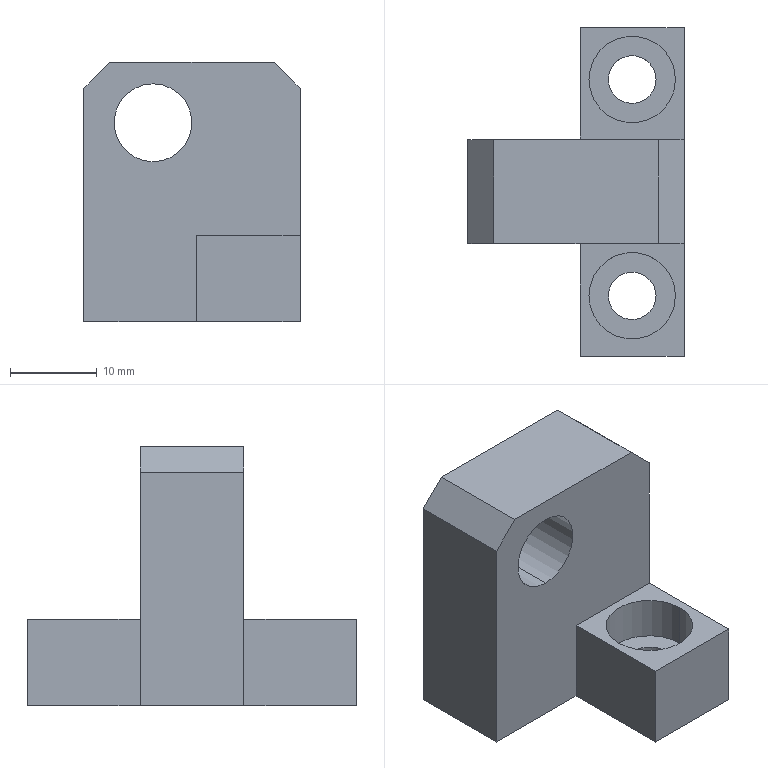Part | STEP file | 11-FG-E00411 | 1 solid | 26 faces | box 25 x 38 x 30 mm | volume 10226 mm3 | plane 16 | cylinder 10 | commonest cylinder face diameters 5.5 x4 10 x4 9 x2
STEP:
#1=CARTESIAN_POINT('',(-25.941,19.216,5.));
#2=VERTEX_POINT('',#1);
#3=CARTESIAN_POINT('',(-15.941,19.216,5.));
#4=VERTEX_POINT('',#3);
#5=CARTESIAN_POINT('',(-20.941,19.216,5.));
#6=DIRECTION('',(0.,0.,1.));
#7=DIRECTION('',(1.,0.,0.));
#8=AXIS2_PLACEMENT_3D('',#5,#6,#7);
#9=CIRCLE('',#8,5.);
#10=EDGE_CURVE('',#2,#4,#9,.T.);
#11=ORIENTED_EDGE('',*,*,#10,.F.);
#12=CARTESIAN_POINT('',(-25.941,19.216,10.));
#13=VERTEX_POINT('',#12);
#14=CARTESIAN_POINT('',(-25.941,19.216,10.));
#15=DIRECTION('',(0.,0.,1.));
#16=VECTOR('',#15,1000.);
#17=LINE('',#14,#16);
#18=EDGE_CURVE('',#2,#13,#17,.T.);
#19=ORIENTED_EDGE('',*,*,#18,.T.);
#20=CARTESIAN_POINT('',(-15.941,19.216,10.));
#21=VERTEX_POINT('',#20);
#22=CARTESIAN_POINT('',(-20.941,19.216,10.));
#23=DIRECTION('',(0.,0.,1.));
#24=DIRECTION('',(1.,0.,0.));
#25=AXIS2_PLACEMENT_3D('',#22,#23,#24);
#26=CIRCLE('',#25,5.);
#27=EDGE_CURVE('',#13,#21,#26,.T.);
#28=ORIENTED_EDGE('',*,*,#27,.T.);
#29=CARTESIAN_POINT('',(-15.941,19.216,10.));
#30=DIRECTION('',(0.,0.,1.));
#31=VECTOR('',#30,1000.);
#32=LINE('',#29,#31);
#33=EDGE_CURVE('',#4,#21,#32,.T.);
#34=ORIENTED_EDGE('',*,*,#33,.F.);
#35=EDGE_LOOP('',(#11,#19,#28,#34));
#36=FACE_OUTER_BOUND('',#35,.T.);
#37=CARTESIAN_POINT('',(-20.941,19.216,10.));
#38=DIRECTION('',(0.,0.,1.));
#39=DIRECTION('',(1.,0.,0.));
#40=AXIS2_PLACEMENT_3D('',#37,#38,#39);
#41=CYLINDRICAL_SURFACE('',#40,5.);
#42=ADVANCED_FACE('',(#36),#41,.F.);
#43=CARTESIAN_POINT('',(-23.691,19.216,0.));
#44=VERTEX_POINT('',#43);
#45=CARTESIAN_POINT('',(-18.191,19.216,0.));
#46=VERTEX_POINT('',#45);
#47=CARTESIAN_POINT('',(-20.941,19.216,0.));
#48=DIRECTION('',(0.,0.,1.));
#49=DIRECTION('',(1.,0.,0.));
#50=AXIS2_PLACEMENT_3D('',#47,#48,#49);
#51=CIRCLE('',#50,2.75);
#52=EDGE_CURVE('',#44,#46,#51,.T.);
#53=ORIENTED_EDGE('',*,*,#52,.F.);
#54=CARTESIAN_POINT('',(-23.691,19.216,5.));
#55=VERTEX_POINT('',#54);
#56=CARTESIAN_POINT('',(-23.691,19.216,10.));
#57=DIRECTION('',(0.,0.,1.));
#58=VECTOR('',#57,1000.);
#59=LINE('',#56,#58);
#60=EDGE_CURVE('',#44,#55,#59,.T.);
#61=ORIENTED_EDGE('',*,*,#60,.T.);
#62=CARTESIAN_POINT('',(-18.191,19.216,5.));
#63=VERTEX_POINT('',#62);
#64=CARTESIAN_POINT('',(-20.941,19.216,5.));
#65=DIRECTION('',(0.,0.,1.));
#66=DIRECTION('',(1.,0.,0.));
#67=AXIS2_PLACEMENT_3D('',#64,#65,#66);
#68=CIRCLE('',#67,2.75);
#69=EDGE_CURVE('',#55,#63,#68,.T.);
#70=ORIENTED_EDGE('',*,*,#69,.T.);
#71=CARTESIAN_POINT('',(-18.191,19.216,10.));
#72=DIRECTION('',(0.,0.,1.));
#73=VECTOR('',#72,1000.);
#74=LINE('',#71,#73);
#75=EDGE_CURVE('',#46,#63,#74,.T.);
#76=ORIENTED_EDGE('',*,*,#75,.F.);
#77=EDGE_LOOP('',(#53,#61,#70,#76));
#78=FACE_OUTER_BOUND('',#77,.T.);
#79=CARTESIAN_POINT('',(-20.941,19.216,10.));
#80=DIRECTION('',(0.,0.,1.));
#81=DIRECTION('',(1.,0.,0.));
#82=AXIS2_PLACEMENT_3D('',#79,#80,#81);
#83=CYLINDRICAL_SURFACE('',#82,2.75);
#84=ADVANCED_FACE('',(#78),#83,.F.);
#85=CARTESIAN_POINT('',(-25.941,-5.784,5.));
#86=VERTEX_POINT('',#85);
#87=CARTESIAN_POINT('',(-15.941,-5.784,5.));
#88=VERTEX_POINT('',#87);
#89=CARTESIAN_POINT('',(-20.941,-5.784,5.));
#90=DIRECTION('',(0.,0.,1.));
#91=DIRECTION('',(1.,0.,0.));
#92=AXIS2_PLACEMENT_3D('',#89,#90,#91);
#93=CIRCLE('',#92,5.);
#94=EDGE_CURVE('',#86,#88,#93,.T.);
#95=ORIENTED_EDGE('',*,*,#94,.F.);
#96=CARTESIAN_POINT('',(-25.941,-5.784,10.));
#97=VERTEX_POINT('',#96);
#98=CARTESIAN_POINT('',(-25.941,-5.784,10.));
#99=DIRECTION('',(0.,0.,1.));
#100=VECTOR('',#99,1000.);
#101=LINE('',#98,#100);
#102=EDGE_CURVE('',#86,#97,#101,.T.);
#103=ORIENTED_EDGE('',*,*,#102,.T.);
#104=CARTESIAN_POINT('',(-15.941,-5.784,10.));
#105=VERTEX_POINT('',#104);
#106=CARTESIAN_POINT('',(-20.941,-5.784,10.));
#107=DIRECTION('',(0.,0.,1.));
#108=DIRECTION('',(1.,0.,0.));
#109=AXIS2_PLACEMENT_3D('',#106,#107,#108);
#110=CIRCLE('',#109,5.);
#111=EDGE_CURVE('',#97,#105,#110,.T.);
#112=ORIENTED_EDGE('',*,*,#111,.T.);
#113=CARTESIAN_POINT('',(-15.941,-5.784,10.));
#114=DIRECTION('',(0.,0.,1.));
#115=VECTOR('',#114,1000.);
#116=LINE('',#113,#115);
#117=EDGE_CURVE('',#88,#105,#116,.T.);
#118=ORIENTED_EDGE('',*,*,#117,.F.);
#119=EDGE_LOOP('',(#95,#103,#112,#118));
#120=FACE_OUTER_BOUND('',#119,.T.);
#121=CARTESIAN_POINT('',(-20.941,-5.784,10.));
#122=DIRECTION('',(0.,0.,1.));
#123=DIRECTION('',(1.,0.,0.));
#124=AXIS2_PLACEMENT_3D('',#121,#122,#123);
#125=CYLINDRICAL_SURFACE('',#124,5.);
#126=ADVANCED_FACE('',(#120),#125,.F.);
#127=CARTESIAN_POINT('',(-23.691,-5.784,0.));
#128=VERTEX_POINT('',#127);
#129=CARTESIAN_POINT('',(-18.191,-5.784,0.));
#130=VERTEX_POINT('',#129);
#131=CARTESIAN_POINT('',(-20.941,-5.784,0.));
#132=DIRECTION('',(0.,0.,1.));
#133=DIRECTION('',(1.,0.,0.));
#134=AXIS2_PLACEMENT_3D('',#131,#132,#133);
#135=CIRCLE('',#134,2.75);
#136=EDGE_CURVE('',#128,#130,#135,.T.);
#137=ORIENTED_EDGE('',*,*,#136,.F.);
#138=CARTESIAN_POINT('',(-23.691,-5.784,5.));
#139=VERTEX_POINT('',#138);
#140=CARTESIAN_POINT('',(-23.691,-5.784,10.));
#141=DIRECTION('',(0.,0.,1.));
#142=VECTOR('',#141,1000.);
#143=LINE('',#140,#142);
#144=EDGE_CURVE('',#128,#139,#143,.T.);
#145=ORIENTED_EDGE('',*,*,#144,.T.);
#146=CARTESIAN_POINT('',(-18.191,-5.784,5.));
#147=VERTEX_POINT('',#146);
#148=CARTESIAN_POINT('',(-20.941,-5.784,5.));
#149=DIRECTION('',(0.,0.,1.));
#150=DIRECTION('',(1.,0.,0.));
#151=AXIS2_PLACEMENT_3D('',#148,#149,#150);
#152=CIRCLE('',#151,2.75);
#153=EDGE_CURVE('',#139,#147,#152,.T.);
#154=ORIENTED_EDGE('',*,*,#153,.T.);
#155=CARTESIAN_POINT('',(-18.191,-5.784,10.));
#156=DIRECTION('',(0.,0.,1.));
#157=VECTOR('',#156,1000.);
#158=LINE('',#155,#157);
#159=EDGE_CURVE('',#130,#147,#158,.T.);
#160=ORIENTED_EDGE('',*,*,#159,.F.);
#161=EDGE_LOOP('',(#137,#145,#154,#160));
#162=FACE_OUTER_BOUND('',#161,.T.);
#163=CARTESIAN_POINT('',(-20.941,-5.784,10.));
#164=DIRECTION('',(0.,0.,1.));
#165=DIRECTION('',(1.,0.,0.));
#166=AXIS2_PLACEMENT_3D('',#163,#164,#165);
#167=CYLINDRICAL_SURFACE('',#166,2.75);
#168=ADVANCED_FACE('',(#162),#167,.F.);
#169=CARTESIAN_POINT('',(-31.941,0.2155,18.5));
#170=VERTEX_POINT('',#169);
#171=CARTESIAN_POINT('',(-31.941,0.2155,27.5));
#172=VERTEX_POINT('',#171);
#173=CARTESIAN_POINT('',(-31.941,0.2155,23.));
#174=DIRECTION('',(0.,1.,0.));
#175=DIRECTION('',(-1.,0.,0.));
#176=AXIS2_PLACEMENT_3D('',#173,#174,#175);
#177=CIRCLE('',#176,4.5);
#178=EDGE_CURVE('',#170,#172,#177,.T.);
#179=ORIENTED_EDGE('',*,*,#178,.F.);
#180=CARTESIAN_POINT('',(-31.941,12.216,18.5));
#181=VERTEX_POINT('',#180);
#182=CARTESIAN_POINT('',(-31.941,12.216,18.5));
#183=DIRECTION('',(0.,1.,0.));
#184=VECTOR('',#183,1000.);
#185=LINE('',#182,#184);
#186=EDGE_CURVE('',#170,#181,#185,.T.);
#187=ORIENTED_EDGE('',*,*,#186,.T.);
#188=CARTESIAN_POINT('',(-31.941,12.216,27.5));
#189=VERTEX_POINT('',#188);
#190=CARTESIAN_POINT('',(-31.941,12.216,23.));
#191=DIRECTION('',(0.,1.,0.));
#192=DIRECTION('',(0.,0.,1.));
#193=AXIS2_PLACEMENT_3D('',#190,#191,#192);
#194=CIRCLE('',#193,4.5);
#195=EDGE_CURVE('',#181,#189,#194,.T.);
#196=ORIENTED_EDGE('',*,*,#195,.T.);
#197=CARTESIAN_POINT('',(-31.941,12.216,27.5));
#198=DIRECTION('',(0.,1.,0.));
#199=VECTOR('',#198,1000.);
#200=LINE('',#197,#199);
#201=EDGE_CURVE('',#172,#189,#200,.T.);
#202=ORIENTED_EDGE('',*,*,#201,.F.);
#203=EDGE_LOOP('',(#179,#187,#196,#202));
#204=FACE_OUTER_BOUND('',#203,.T.);
#205=CARTESIAN_POINT('',(-31.941,12.216,23.));
#206=DIRECTION('',(0.,1.,0.));
#207=DIRECTION('',(0.,0.,1.));
#208=AXIS2_PLACEMENT_3D('',#205,#206,#207);
#209=CYLINDRICAL_SURFACE('',#208,4.5);
#210=ADVANCED_FACE('',(#204),#209,.F.);
#211=CARTESIAN_POINT('',(-14.941,0.2155,10.));
#212=VERTEX_POINT('',#211);
#213=CARTESIAN_POINT('',(-26.941,0.2155,10.));
#214=VERTEX_POINT('',#213);
#215=CARTESIAN_POINT('',(-39.941,0.2155,10.));
#216=DIRECTION('',(-1.,0.,0.));
#217=VECTOR('',#216,1000.);
#218=LINE('',#215,#217);
#219=EDGE_CURVE('',#212,#214,#218,.T.);
#220=ORIENTED_EDGE('',*,*,#219,.T.);
#221=CARTESIAN_POINT('',(-26.941,-12.784,10.));
#222=VERTEX_POINT('',#221);
#223=CARTESIAN_POINT('',(-26.941,-24.784,10.));
#224=DIRECTION('',(0.,1.,0.));
#225=VECTOR('',#224,1000.);
#226=LINE('',#223,#225);
#227=EDGE_CURVE('',#222,#214,#226,.T.);
#228=ORIENTED_EDGE('',*,*,#227,.F.);
#229=CARTESIAN_POINT('',(-14.941,-12.784,10.));
#230=VERTEX_POINT('',#229);
#231=CARTESIAN_POINT('',(-14.941,-12.784,10.));
#232=DIRECTION('',(-1.,0.,0.));
#233=VECTOR('',#232,1000.);
#234=LINE('',#231,#233);
#235=EDGE_CURVE('',#230,#222,#234,.T.);
#236=ORIENTED_EDGE('',*,*,#235,.F.);
#237=CARTESIAN_POINT('',(-14.941,-24.784,10.));
#238=DIRECTION('',(0.,1.,0.));
#239=VECTOR('',#238,1000.);
#240=LINE('',#237,#239);
#241=EDGE_CURVE('',#230,#212,#240,.T.);
#242=ORIENTED_EDGE('',*,*,#241,.T.);
#243=EDGE_LOOP('',(#220,#228,#236,#242));
#244=FACE_OUTER_BOUND('',#243,.T.);
#245=CARTESIAN_POINT('',(-20.941,-5.784,10.));
#246=DIRECTION('',(0.,0.,1.));
#247=DIRECTION('',(1.,0.,0.));
#248=AXIS2_PLACEMENT_3D('',#245,#246,#247);
#249=CIRCLE('',#248,5.);
#250=EDGE_CURVE('',#105,#97,#249,.T.);
#251=ORIENTED_EDGE('',*,*,#250,.F.);
#252=ORIENTED_EDGE('',*,*,#111,.F.);
#253=EDGE_LOOP('',(#251,#252));
#254=FACE_BOUND('',#253,.T.);
#255=CARTESIAN_POINT('',(-39.941,0.2155,10.));
#256=DIRECTION('',(0.,0.,-1.));
#257=DIRECTION('',(-1.,0.,0.));
#258=AXIS2_PLACEMENT_3D('',#255,#256,#257);
#259=PLANE('',#258);
#260=ADVANCED_FACE('',(#244,#254),#259,.F.);
#261=CARTESIAN_POINT('',(-36.941,12.216,30.));
#262=VERTEX_POINT('',#261);
#263=CARTESIAN_POINT('',(-17.941,12.216,30.));
#264=VERTEX_POINT('',#263);
#265=CARTESIAN_POINT('',(-39.941,12.216,30.));
#266=DIRECTION('',(1.,0.,0.));
#267=VECTOR('',#266,1000.);
#268=LINE('',#265,#267);
#269=EDGE_CURVE('',#262,#264,#268,.T.);
#270=ORIENTED_EDGE('',*,*,#269,.T.);
#271=CARTESIAN_POINT('',(-14.941,12.216,27.));
#272=VERTEX_POINT('',#271);
#273=CARTESIAN_POINT('',(-17.941,12.216,30.));
#274=DIRECTION('',(0.7071,0.,-0.7071));
#275=VECTOR('',#274,1000.);
#276=LINE('',#273,#275);
#277=EDGE_CURVE('',#264,#272,#276,.T.);
#278=ORIENTED_EDGE('',*,*,#277,.T.);
#279=CARTESIAN_POINT('',(-14.941,12.216,10.));
#280=VERTEX_POINT('',#279);
#281=CARTESIAN_POINT('',(-14.941,12.216,10.));
#282=DIRECTION('',(0.,0.,1.));
#283=VECTOR('',#282,1000.);
#284=LINE('',#281,#283);
#285=EDGE_CURVE('',#280,#272,#284,.T.);
#286=ORIENTED_EDGE('',*,*,#285,.F.);
#287=CARTESIAN_POINT('',(-26.941,12.216,10.));
#288=VERTEX_POINT('',#287);
#289=CARTESIAN_POINT('',(-39.941,12.216,10.));
#290=DIRECTION('',(1.,0.,0.));
#291=VECTOR('',#290,1000.);
#292=LINE('',#289,#291);
#293=EDGE_CURVE('',#288,#280,#292,.T.);
#294=ORIENTED_EDGE('',*,*,#293,.F.);
#295=CARTESIAN_POINT('',(-26.941,12.216,0.));
#296=VERTEX_POINT('',#295);
#297=CARTESIAN_POINT('',(-26.941,12.216,0.));
#298=DIRECTION('',(0.,0.,1.));
#299=VECTOR('',#298,1000.);
#300=LINE('',#297,#299);
#301=EDGE_CURVE('',#296,#288,#300,.T.);
#302=ORIENTED_EDGE('',*,*,#301,.F.);
#303=CARTESIAN_POINT('',(-39.941,12.216,0.));
#304=VERTEX_POINT('',#303);
#305=CARTESIAN_POINT('',(-39.941,12.216,0.));
#306=DIRECTION('',(1.,0.,0.));
#307=VECTOR('',#306,1000.);
#308=LINE('',#305,#307);
#309=EDGE_CURVE('',#304,#296,#308,.T.);
#310=ORIENTED_EDGE('',*,*,#309,.F.);
#311=CARTESIAN_POINT('',(-39.941,12.216,27.));
#312=VERTEX_POINT('',#311);
#313=CARTESIAN_POINT('',(-39.941,12.216,10.));
#314=DIRECTION('',(0.,0.,1.));
#315=VECTOR('',#314,1000.);
#316=LINE('',#313,#315);
#317=EDGE_CURVE('',#304,#312,#316,.T.);
#318=ORIENTED_EDGE('',*,*,#317,.T.);
#319=CARTESIAN_POINT('',(-36.941,12.216,30.));
#320=DIRECTION('',(0.7071,0.,0.7071));
#321=VECTOR('',#320,1000.);
#322=LINE('',#319,#321);
#323=EDGE_CURVE('',#312,#262,#322,.T.);
#324=ORIENTED_EDGE('',*,*,#323,.T.);
#325=EDGE_LOOP('',(#270,#278,#286,#294,#302,#310,#318,#324));
#326=FACE_OUTER_BOUND('',#325,.T.);
#327=CARTESIAN_POINT('',(-31.941,12.216,23.));
#328=DIRECTION('',(0.,1.,0.));
#329=DIRECTION('',(0.,0.,1.));
#330=AXIS2_PLACEMENT_3D('',#327,#328,#329);
#331=CIRCLE('',#330,4.5);
#332=EDGE_CURVE('',#189,#181,#331,.T.);
#333=ORIENTED_EDGE('',*,*,#332,.F.);
#334=ORIENTED_EDGE('',*,*,#195,.F.);
#335=EDGE_LOOP('',(#333,#334));
#336=FACE_BOUND('',#335,.T.);
#337=CARTESIAN_POINT('',(-39.941,12.216,10.));
#338=DIRECTION('',(0.,-1.,0.));
#339=DIRECTION('',(0.,0.,-1.));
#340=AXIS2_PLACEMENT_3D('',#337,#338,#339);
#341=PLANE('',#340);
#342=ADVANCED_FACE('',(#326,#336),#341,.F.);
#343=CARTESIAN_POINT('',(-14.941,25.216,0.));
#344=VERTEX_POINT('',#343);
#345=CARTESIAN_POINT('',(-26.941,25.216,0.));
#346=VERTEX_POINT('',#345);
#347=CARTESIAN_POINT('',(-39.941,25.216,0.));
#348=DIRECTION('',(-1.,0.,0.));
#349=VECTOR('',#348,1000.);
#350=LINE('',#347,#349);
#351=EDGE_CURVE('',#344,#346,#350,.T.);
#352=ORIENTED_EDGE('',*,*,#351,.T.);
#353=CARTESIAN_POINT('',(-26.941,25.216,10.));
#354=VERTEX_POINT('',#353);
#355=CARTESIAN_POINT('',(-26.941,25.216,0.));
#356=DIRECTION('',(0.,0.,1.));
#357=VECTOR('',#356,1000.);
#358=LINE('',#355,#357);
#359=EDGE_CURVE('',#346,#354,#358,.T.);
#360=ORIENTED_EDGE('',*,*,#359,.T.);
#361=CARTESIAN_POINT('',(-14.941,25.216,10.));
#362=VERTEX_POINT('',#361);
#363=CARTESIAN_POINT('',(-39.941,25.216,10.));
#364=DIRECTION('',(-1.,0.,0.));
#365=VECTOR('',#364,1000.);
#366=LINE('',#363,#365);
#367=EDGE_CURVE('',#362,#354,#366,.T.);
#368=ORIENTED_EDGE('',*,*,#367,.F.);
#369=CARTESIAN_POINT('',(-14.941,25.216,30.));
#370=DIRECTION('',(0.,0.,-1.));
#371=VECTOR('',#370,1000.);
#372=LINE('',#369,#371);
#373=EDGE_CURVE('',#362,#344,#372,.T.);
#374=ORIENTED_EDGE('',*,*,#373,.T.);
#375=EDGE_LOOP('',(#352,#360,#368,#374));
#376=FACE_OUTER_BOUND('',#375,.T.);
#377=CARTESIAN_POINT('',(-39.941,25.216,30.));
#378=DIRECTION('',(0.,-1.,0.));
#379=DIRECTION('',(0.,0.,-1.));
#380=AXIS2_PLACEMENT_3D('',#377,#378,#379);
#381=PLANE('',#380);
#382=ADVANCED_FACE('',(#376),#381,.F.);
#383=CARTESIAN_POINT('',(-39.941,0.2155,0.));
#384=VERTEX_POINT('',#383);
#385=CARTESIAN_POINT('',(-39.941,0.2155,27.));
#386=VERTEX_POINT('',#385);
#387=CARTESIAN_POINT('',(-39.941,0.2155,10.));
#388=DIRECTION('',(0.,0.,1.));
#389=VECTOR('',#388,1000.);
#390=LINE('',#387,#389);
#391=EDGE_CURVE('',#384,#386,#390,.T.);
#392=ORIENTED_EDGE('',*,*,#391,.T.);
#393=CARTESIAN_POINT('',(-39.941,12.216,27.));
#394=DIRECTION('',(0.,1.,0.));
#395=VECTOR('',#394,1000.);
#396=LINE('',#393,#395);
#397=EDGE_CURVE('',#386,#312,#396,.T.);
#398=ORIENTED_EDGE('',*,*,#397,.T.);
#399=ORIENTED_EDGE('',*,*,#317,.F.);
#400=CARTESIAN_POINT('',(-39.941,25.216,0.));
#401=DIRECTION('',(0.,-1.,0.));
#402=VECTOR('',#401,1000.);
#403=LINE('',#400,#402);
#404=EDGE_CURVE('',#304,#384,#403,.T.);
#405=ORIENTED_EDGE('',*,*,#404,.T.);
#406=EDGE_LOOP('',(#392,#398,#399,#405));
#407=FACE_OUTER_BOUND('',#406,.T.);
#408=CARTESIAN_POINT('',(-39.941,25.216,30.));
#409=DIRECTION('',(1.,0.,0.));
#410=DIRECTION('',(0.,1.,0.));
#411=AXIS2_PLACEMENT_3D('',#408,#409,#410);
#412=PLANE('',#411);
#413=ADVANCED_FACE('',(#407),#412,.F.);
#414=ORIENTED_EDGE('',*,*,#285,.T.);
#415=CARTESIAN_POINT('',(-14.941,0.2155,27.));
#416=VERTEX_POINT('',#415);
#417=CARTESIAN_POINT('',(-14.941,0.2155,27.));
#418=DIRECTION('',(0.,-1.,0.));
#419=VECTOR('',#418,1000.);
#420=LINE('',#417,#419);
#421=EDGE_CURVE('',#272,#416,#420,.T.);
#422=ORIENTED_EDGE('',*,*,#421,.T.);
#423=CARTESIAN_POINT('',(-14.941,0.2155,10.));
#424=DIRECTION('',(0.,0.,1.));
#425=VECTOR('',#424,1000.);
#426=LINE('',#423,#425);
#427=EDGE_CURVE('',#212,#416,#426,.T.);
#428=ORIENTED_EDGE('',*,*,#427,.F.);
#429=ORIENTED_EDGE('',*,*,#241,.F.);
#430=CARTESIAN_POINT('',(-14.941,-12.784,0.));
#431=VERTEX_POINT('',#430);
#432=CARTESIAN_POINT('',(-14.941,-12.784,0.));
#433=DIRECTION('',(0.,0.,1.));
#434=VECTOR('',#433,1000.);
#435=LINE('',#432,#434);
#436=EDGE_CURVE('',#431,#230,#435,.T.);
#437=ORIENTED_EDGE('',*,*,#436,.F.);
#438=CARTESIAN_POINT('',(-14.941,25.216,0.));
#439=DIRECTION('',(0.,1.,0.));
#440=VECTOR('',#439,1000.);
#441=LINE('',#438,#440);
#442=EDGE_CURVE('',#431,#344,#441,.T.);
#443=ORIENTED_EDGE('',*,*,#442,.T.);
#444=ORIENTED_EDGE('',*,*,#373,.F.);
#445=CARTESIAN_POINT('',(-14.941,25.216,10.));
#446=DIRECTION('',(0.,1.,0.));
#447=VECTOR('',#446,1000.);
#448=LINE('',#445,#447);
#449=EDGE_CURVE('',#280,#362,#448,.T.);
#450=ORIENTED_EDGE('',*,*,#449,.F.);
#451=EDGE_LOOP('',(#414,#422,#428,#429,#437,#443,#444,#450));
#452=FACE_OUTER_BOUND('',#451,.T.);
#453=CARTESIAN_POINT('',(-14.941,25.216,30.));
#454=DIRECTION('',(-1.,0.,0.));
#455=DIRECTION('',(0.,-1.,0.));
#456=AXIS2_PLACEMENT_3D('',#453,#454,#455);
#457=PLANE('',#456);
#458=ADVANCED_FACE('',(#452),#457,.F.);
#459=CARTESIAN_POINT('',(-17.941,0.2155,30.));
#460=VERTEX_POINT('',#459);
#461=CARTESIAN_POINT('',(-36.941,0.2155,30.));
#462=VERTEX_POINT('',#461);
#463=CARTESIAN_POINT('',(-39.941,0.2155,30.));
#464=DIRECTION('',(-1.,0.,0.));
#465=VECTOR('',#464,1000.);
#466=LINE('',#463,#465);
#467=EDGE_CURVE('',#460,#462,#466,.T.);
#468=ORIENTED_EDGE('',*,*,#467,.F.);
#469=CARTESIAN_POINT('',(-17.941,12.216,30.));
#470=DIRECTION('',(0.,1.,0.));
#471=VECTOR('',#470,1000.);
#472=LINE('',#469,#471);
#473=EDGE_CURVE('',#460,#264,#472,.T.);
#474=ORIENTED_EDGE('',*,*,#473,.T.);
#475=ORIENTED_EDGE('',*,*,#269,.F.);
#476=CARTESIAN_POINT('',(-36.941,0.2155,30.));
#477=DIRECTION('',(0.,-1.,0.));
#478=VECTOR('',#477,1000.);
#479=LINE('',#476,#478);
#480=EDGE_CURVE('',#262,#462,#479,.T.);
#481=ORIENTED_EDGE('',*,*,#480,.T.);
#482=EDGE_LOOP('',(#468,#474,#475,#481));
#483=FACE_OUTER_BOUND('',#482,.T.);
#484=CARTESIAN_POINT('',(-39.941,-24.784,30.));
#485=DIRECTION('',(0.,0.,1.));
#486=DIRECTION('',(1.,0.,0.));
#487=AXIS2_PLACEMENT_3D('',#484,#485,#486);
#488=PLANE('',#487);
#489=ADVANCED_FACE('',(#483),#488,.T.);
#490=CARTESIAN_POINT('',(-20.941,19.216,0.));
#491=DIRECTION('',(0.,0.,1.));
#492=DIRECTION('',(1.,0.,0.));
#493=AXIS2_PLACEMENT_3D('',#490,#491,#492);
#494=CIRCLE('',#493,2.75);
#495=EDGE_CURVE('',#46,#44,#494,.T.);
#496=ORIENTED_EDGE('',*,*,#495,.T.);
#497=ORIENTED_EDGE('',*,*,#52,.T.);
#498=EDGE_LOOP('',(#496,#497));
#499=FACE_BOUND('',#498,.T.);
#500=CARTESIAN_POINT('',(-20.941,-5.784,0.));
#501=DIRECTION('',(0.,0.,1.));
#502=DIRECTION('',(1.,0.,0.));
#503=AXIS2_PLACEMENT_3D('',#500,#501,#502);
#504=CIRCLE('',#503,2.75);
#505=EDGE_CURVE('',#130,#128,#504,.T.);
#506=ORIENTED_EDGE('',*,*,#505,.T.);
#507=ORIENTED_EDGE('',*,*,#136,.T.);
#508=EDGE_LOOP('',(#506,#507));
#509=FACE_BOUND('',#508,.T.);
#510=CARTESIAN_POINT('',(-26.941,-12.784,0.));
#511=VERTEX_POINT('',#510);
#512=CARTESIAN_POINT('',(-26.941,0.2155,0.));
#513=VERTEX_POINT('',#512);
#514=CARTESIAN_POINT('',(-26.941,-24.784,0.));
#515=DIRECTION('',(0.,1.,0.));
#516=VECTOR('',#515,1000.);
#517=LINE('',#514,#516);
#518=EDGE_CURVE('',#511,#513,#517,.T.);
#519=ORIENTED_EDGE('',*,*,#518,.T.);
#520=CARTESIAN_POINT('',(-39.941,0.2155,0.));
#521=DIRECTION('',(-1.,0.,0.));
#522=VECTOR('',#521,1000.);
#523=LINE('',#520,#522);
#524=EDGE_CURVE('',#513,#384,#523,.T.);
#525=ORIENTED_EDGE('',*,*,#524,.T.);
#526=ORIENTED_EDGE('',*,*,#404,.F.);
#527=ORIENTED_EDGE('',*,*,#309,.T.);
#528=CARTESIAN_POINT('',(-26.941,25.216,0.));
#529=DIRECTION('',(0.,1.,0.));
#530=VECTOR('',#529,1000.);
#531=LINE('',#528,#530);
#532=EDGE_CURVE('',#296,#346,#531,.T.);
#533=ORIENTED_EDGE('',*,*,#532,.T.);
#534=ORIENTED_EDGE('',*,*,#351,.F.);
#535=ORIENTED_EDGE('',*,*,#442,.F.);
#536=CARTESIAN_POINT('',(-14.941,-12.784,0.));
#537=DIRECTION('',(-1.,0.,0.));
#538=VECTOR('',#537,1000.);
#539=LINE('',#536,#538);
#540=EDGE_CURVE('',#431,#511,#539,.T.);
#541=ORIENTED_EDGE('',*,*,#540,.T.);
#542=EDGE_LOOP('',(#519,#525,#526,#527,#533,#534,#535,#541));
#543=FACE_OUTER_BOUND('',#542,.T.);
#544=CARTESIAN_POINT('',(-39.941,-24.784,0.));
#545=DIRECTION('',(0.,0.,1.));
#546=DIRECTION('',(1.,0.,0.));
#547=AXIS2_PLACEMENT_3D('',#544,#545,#546);
#548=PLANE('',#547);
#549=ADVANCED_FACE('',(#499,#509,#543),#548,.F.);
#550=CARTESIAN_POINT('',(-20.941,19.216,10.));
#551=DIRECTION('',(0.,0.,1.));
#552=DIRECTION('',(1.,0.,0.));
#553=AXIS2_PLACEMENT_3D('',#550,#551,#552);
#554=CIRCLE('',#553,5.);
#555=EDGE_CURVE('',#21,#13,#554,.T.);
#556=ORIENTED_EDGE('',*,*,#555,.F.);
#557=ORIENTED_EDGE('',*,*,#27,.F.);
#558=EDGE_LOOP('',(#556,#557));
#559=FACE_BOUND('',#558,.T.);
#560=CARTESIAN_POINT('',(-26.941,25.216,10.));
#561=DIRECTION('',(0.,1.,0.));
#562=VECTOR('',#561,1000.);
#563=LINE('',#560,#562);
#564=EDGE_CURVE('',#288,#354,#563,.T.);
#565=ORIENTED_EDGE('',*,*,#564,.F.);
#566=ORIENTED_EDGE('',*,*,#293,.T.);
#567=ORIENTED_EDGE('',*,*,#449,.T.);
#568=ORIENTED_EDGE('',*,*,#367,.T.);
#569=EDGE_LOOP('',(#565,#566,#567,#568));
#570=FACE_OUTER_BOUND('',#569,.T.);
#571=CARTESIAN_POINT('',(-39.941,12.216,10.));
#572=DIRECTION('',(0.,0.,1.));
#573=DIRECTION('',(1.,0.,0.));
#574=AXIS2_PLACEMENT_3D('',#571,#572,#573);
#575=PLANE('',#574);
#576=ADVANCED_FACE('',(#559,#570),#575,.T.);
#577=CARTESIAN_POINT('',(-31.941,0.2155,23.));
#578=DIRECTION('',(0.,1.,0.));
#579=DIRECTION('',(-1.,0.,0.));
#580=AXIS2_PLACEMENT_3D('',#577,#578,#579);
#581=CIRCLE('',#580,4.5);
#582=EDGE_CURVE('',#172,#170,#581,.T.);
#583=ORIENTED_EDGE('',*,*,#582,.T.);
#584=ORIENTED_EDGE('',*,*,#178,.T.);
#585=EDGE_LOOP('',(#583,#584));
#586=FACE_BOUND('',#585,.T.);
#587=ORIENTED_EDGE('',*,*,#427,.T.);
#588=CARTESIAN_POINT('',(-17.941,0.2155,30.));
#589=DIRECTION('',(-0.7071,0.,0.7071));
#590=VECTOR('',#589,1000.);
#591=LINE('',#588,#590);
#592=EDGE_CURVE('',#416,#460,#591,.T.);
#593=ORIENTED_EDGE('',*,*,#592,.T.);
#594=ORIENTED_EDGE('',*,*,#467,.T.);
#595=CARTESIAN_POINT('',(-36.941,0.2155,30.));
#596=DIRECTION('',(-0.7071,0.,-0.7071));
#597=VECTOR('',#596,1000.);
#598=LINE('',#595,#597);
#599=EDGE_CURVE('',#462,#386,#598,.T.);
#600=ORIENTED_EDGE('',*,*,#599,.T.);
#601=ORIENTED_EDGE('',*,*,#391,.F.);
#602=ORIENTED_EDGE('',*,*,#524,.F.);
#603=CARTESIAN_POINT('',(-26.941,0.2155,0.));
#604=DIRECTION('',(0.,0.,1.));
#605=VECTOR('',#604,1000.);
#606=LINE('',#603,#605);
#607=EDGE_CURVE('',#513,#214,#606,.T.);
#608=ORIENTED_EDGE('',*,*,#607,.T.);
#609=ORIENTED_EDGE('',*,*,#219,.F.);
#610=EDGE_LOOP('',(#587,#593,#594,#600,#601,#602,#608,#609));
#611=FACE_OUTER_BOUND('',#610,.T.);
#612=CARTESIAN_POINT('',(-39.941,0.2155,10.));
#613=DIRECTION('',(0.,1.,0.));
#614=DIRECTION('',(-1.,0.,0.));
#615=AXIS2_PLACEMENT_3D('',#612,#613,#614);
#616=PLANE('',#615);
#617=ADVANCED_FACE('',(#586,#611),#616,.F.);
#618=ORIENTED_EDGE('',*,*,#186,.F.);
#619=ORIENTED_EDGE('',*,*,#582,.F.);
#620=ORIENTED_EDGE('',*,*,#201,.T.);
#621=ORIENTED_EDGE('',*,*,#332,.T.);
#622=EDGE_LOOP('',(#618,#619,#620,#621));
#623=FACE_OUTER_BOUND('',#622,.T.);
#624=CARTESIAN_POINT('',(-31.941,12.216,23.));
#625=DIRECTION('',(0.,1.,0.));
#626=DIRECTION('',(0.,0.,1.));
#627=AXIS2_PLACEMENT_3D('',#624,#625,#626);
#628=CYLINDRICAL_SURFACE('',#627,4.5);
#629=ADVANCED_FACE('',(#623),#628,.F.);
#630=ORIENTED_EDGE('',*,*,#564,.T.);
#631=ORIENTED_EDGE('',*,*,#359,.F.);
#632=ORIENTED_EDGE('',*,*,#532,.F.);
#633=ORIENTED_EDGE('',*,*,#301,.T.);
#634=EDGE_LOOP('',(#630,#631,#632,#633));
#635=FACE_OUTER_BOUND('',#634,.T.);
#636=CARTESIAN_POINT('',(-26.941,25.216,0.));
#637=DIRECTION('',(1.,0.,0.));
#638=DIRECTION('',(0.,1.,0.));
#639=AXIS2_PLACEMENT_3D('',#636,#637,#638);
#640=PLANE('',#639);
#641=ADVANCED_FACE('',(#635),#640,.F.);
#642=ORIENTED_EDGE('',*,*,#235,.T.);
#643=CARTESIAN_POINT('',(-26.941,-12.784,0.));
#644=DIRECTION('',(0.,0.,-1.));
#645=VECTOR('',#644,1000.);
#646=LINE('',#643,#645);
#647=EDGE_CURVE('',#222,#511,#646,.T.);
#648=ORIENTED_EDGE('',*,*,#647,.T.);
#649=ORIENTED_EDGE('',*,*,#540,.F.);
#650=ORIENTED_EDGE('',*,*,#436,.T.);
#651=EDGE_LOOP('',(#642,#648,#649,#650));
#652=FACE_OUTER_BOUND('',#651,.T.);
#653=CARTESIAN_POINT('',(-14.941,-12.784,0.));
#654=DIRECTION('',(0.,1.,0.));
#655=DIRECTION('',(-1.,0.,0.));
#656=AXIS2_PLACEMENT_3D('',#653,#654,#655);
#657=PLANE('',#656);
#658=ADVANCED_FACE('',(#652),#657,.F.);
#659=ORIENTED_EDGE('',*,*,#144,.F.);
#660=ORIENTED_EDGE('',*,*,#505,.F.);
#661=ORIENTED_EDGE('',*,*,#159,.T.);
#662=CARTESIAN_POINT('',(-20.941,-5.784,5.));
#663=DIRECTION('',(0.,0.,1.));
#664=DIRECTION('',(1.,0.,0.));
#665=AXIS2_PLACEMENT_3D('',#662,#663,#664);
#666=CIRCLE('',#665,2.75);
#667=EDGE_CURVE('',#147,#139,#666,.T.);
#668=ORIENTED_EDGE('',*,*,#667,.T.);
#669=EDGE_LOOP('',(#659,#660,#661,#668));
#670=FACE_OUTER_BOUND('',#669,.T.);
#671=CARTESIAN_POINT('',(-20.941,-5.784,10.));
#672=DIRECTION('',(0.,0.,1.));
#673=DIRECTION('',(1.,0.,0.));
#674=AXIS2_PLACEMENT_3D('',#671,#672,#673);
#675=CYLINDRICAL_SURFACE('',#674,2.75);
#676=ADVANCED_FACE('',(#670),#675,.F.);
#677=ORIENTED_EDGE('',*,*,#667,.F.);
#678=ORIENTED_EDGE('',*,*,#153,.F.);
#679=EDGE_LOOP('',(#677,#678));
#680=FACE_BOUND('',#679,.T.);
#681=CARTESIAN_POINT('',(-20.941,-5.784,5.));
#682=DIRECTION('',(0.,0.,1.));
#683=DIRECTION('',(1.,0.,0.));
#684=AXIS2_PLACEMENT_3D('',#681,#682,#683);
#685=CIRCLE('',#684,5.);
#686=EDGE_CURVE('',#88,#86,#685,.T.);
#687=ORIENTED_EDGE('',*,*,#686,.T.);
#688=ORIENTED_EDGE('',*,*,#94,.T.);
#689=EDGE_LOOP('',(#687,#688));
#690=FACE_OUTER_BOUND('',#689,.T.);
#691=CARTESIAN_POINT('',(-18.191,-5.784,5.));
#692=DIRECTION('',(0.,0.,-1.));
#693=DIRECTION('',(-1.,0.,0.));
#694=AXIS2_PLACEMENT_3D('',#691,#692,#693);
#695=PLANE('',#694);
#696=ADVANCED_FACE('',(#680,#690),#695,.F.);
#697=ORIENTED_EDGE('',*,*,#102,.F.);
#698=ORIENTED_EDGE('',*,*,#686,.F.);
#699=ORIENTED_EDGE('',*,*,#117,.T.);
#700=ORIENTED_EDGE('',*,*,#250,.T.);
#701=EDGE_LOOP('',(#697,#698,#699,#700));
#702=FACE_OUTER_BOUND('',#701,.T.);
#703=CARTESIAN_POINT('',(-20.941,-5.784,10.));
#704=DIRECTION('',(0.,0.,1.));
#705=DIRECTION('',(1.,0.,0.));
#706=AXIS2_PLACEMENT_3D('',#703,#704,#705);
#707=CYLINDRICAL_SURFACE('',#706,5.);
#708=ADVANCED_FACE('',(#702),#707,.F.);
#709=ORIENTED_EDGE('',*,*,#60,.F.);
#710=ORIENTED_EDGE('',*,*,#495,.F.);
#711=ORIENTED_EDGE('',*,*,#75,.T.);
#712=CARTESIAN_POINT('',(-20.941,19.216,5.));
#713=DIRECTION('',(0.,0.,1.));
#714=DIRECTION('',(1.,0.,0.));
#715=AXIS2_PLACEMENT_3D('',#712,#713,#714);
#716=CIRCLE('',#715,2.75);
#717=EDGE_CURVE('',#63,#55,#716,.T.);
#718=ORIENTED_EDGE('',*,*,#717,.T.);
#719=EDGE_LOOP('',(#709,#710,#711,#718));
#720=FACE_OUTER_BOUND('',#719,.T.);
#721=CARTESIAN_POINT('',(-20.941,19.216,10.));
#722=DIRECTION('',(0.,0.,1.));
#723=DIRECTION('',(1.,0.,0.));
#724=AXIS2_PLACEMENT_3D('',#721,#722,#723);
#725=CYLINDRICAL_SURFACE('',#724,2.75);
#726=ADVANCED_FACE('',(#720),#725,.F.);
#727=ORIENTED_EDGE('',*,*,#717,.F.);
#728=ORIENTED_EDGE('',*,*,#69,.F.);
#729=EDGE_LOOP('',(#727,#728));
#730=FACE_BOUND('',#729,.T.);
#731=CARTESIAN_POINT('',(-20.941,19.216,5.));
#732=DIRECTION('',(0.,0.,1.));
#733=DIRECTION('',(1.,0.,0.));
#734=AXIS2_PLACEMENT_3D('',#731,#732,#733);
#735=CIRCLE('',#734,5.);
#736=EDGE_CURVE('',#4,#2,#735,.T.);
#737=ORIENTED_EDGE('',*,*,#736,.T.);
#738=ORIENTED_EDGE('',*,*,#10,.T.);
#739=EDGE_LOOP('',(#737,#738));
#740=FACE_OUTER_BOUND('',#739,.T.);
#741=CARTESIAN_POINT('',(-18.191,19.216,5.));
#742=DIRECTION('',(0.,0.,-1.));
#743=DIRECTION('',(-1.,0.,0.));
#744=AXIS2_PLACEMENT_3D('',#741,#742,#743);
#745=PLANE('',#744);
#746=ADVANCED_FACE('',(#730,#740),#745,.F.);
#747=ORIENTED_EDGE('',*,*,#18,.F.);
#748=ORIENTED_EDGE('',*,*,#736,.F.);
#749=ORIENTED_EDGE('',*,*,#33,.T.);
#750=ORIENTED_EDGE('',*,*,#555,.T.);
#751=EDGE_LOOP('',(#747,#748,#749,#750));
#752=FACE_OUTER_BOUND('',#751,.T.);
#753=CARTESIAN_POINT('',(-20.941,19.216,10.));
#754=DIRECTION('',(0.,0.,1.));
#755=DIRECTION('',(1.,0.,0.));
#756=AXIS2_PLACEMENT_3D('',#753,#754,#755);
#757=CYLINDRICAL_SURFACE('',#756,5.);
#758=ADVANCED_FACE('',(#752),#757,.F.);
#759=ORIENTED_EDGE('',*,*,#592,.F.);
#760=ORIENTED_EDGE('',*,*,#421,.F.);
#761=ORIENTED_EDGE('',*,*,#277,.F.);
#762=ORIENTED_EDGE('',*,*,#473,.F.);
#763=EDGE_LOOP('',(#759,#760,#761,#762));
#764=FACE_OUTER_BOUND('',#763,.T.);
#765=CARTESIAN_POINT('',(-17.941,-24.784,30.));
#766=DIRECTION('',(0.7071,0.,0.7071));
#767=DIRECTION('',(0.7071,0.,-0.7071));
#768=AXIS2_PLACEMENT_3D('',#765,#766,#767);
#769=PLANE('',#768);
#770=ADVANCED_FACE('',(#764),#769,.T.);
#771=ORIENTED_EDGE('',*,*,#323,.F.);
#772=ORIENTED_EDGE('',*,*,#397,.F.);
#773=ORIENTED_EDGE('',*,*,#599,.F.);
#774=ORIENTED_EDGE('',*,*,#480,.F.);
#775=EDGE_LOOP('',(#771,#772,#773,#774));
#776=FACE_OUTER_BOUND('',#775,.T.);
#777=CARTESIAN_POINT('',(-36.941,-24.784,30.));
#778=DIRECTION('',(-0.7071,0.,0.7071));
#779=DIRECTION('',(0.7071,0.,0.7071));
#780=AXIS2_PLACEMENT_3D('',#777,#778,#779);
#781=PLANE('',#780);
#782=ADVANCED_FACE('',(#776),#781,.T.);
#783=ORIENTED_EDGE('',*,*,#227,.T.);
#784=ORIENTED_EDGE('',*,*,#607,.F.);
#785=ORIENTED_EDGE('',*,*,#518,.F.);
#786=ORIENTED_EDGE('',*,*,#647,.F.);
#787=EDGE_LOOP('',(#783,#784,#785,#786));
#788=FACE_OUTER_BOUND('',#787,.T.);
#789=CARTESIAN_POINT('',(-26.941,-24.784,0.));
#790=DIRECTION('',(1.,0.,0.));
#791=DIRECTION('',(0.,0.,-1.));
#792=AXIS2_PLACEMENT_3D('',#789,#790,#791);
#793=PLANE('',#792);
#794=ADVANCED_FACE('',(#788),#793,.F.);
#795=CLOSED_SHELL('',(#42,#84,#126,#168,#210,#260,#342,#382,#413,#458,#489,#549,#576,#617,#629,#641,#658,#676,#696,#708,#726,#746,#758,#770,#782,#794));
#796=MANIFOLD_SOLID_BREP('',#795);
#797=CARTESIAN_POINT('',(0.,0.,0.));
#798=DIRECTION('',(0.,0.,1.));
#799=DIRECTION('',(1.,0.,0.));
#800=AXIS2_PLACEMENT_3D('',#797,#798,#799);
#801=(LENGTH_UNIT()NAMED_UNIT(*)SI_UNIT(.MILLI.,.METRE.));
#802=UNCERTAINTY_MEASURE_WITH_UNIT(LENGTH_MEASURE(0.00001),#801,'','');
#803=(NAMED_UNIT(*)PLANE_ANGLE_UNIT()SI_UNIT($,.RADIAN.));
#804=(NAMED_UNIT(*)SI_UNIT($,.STERADIAN.)SOLID_ANGLE_UNIT());
#805=(GEOMETRIC_REPRESENTATION_CONTEXT(3)GLOBAL_UNCERTAINTY_ASSIGNED_CONTEXT((#802))GLOBAL_UNIT_ASSIGNED_CONTEXT((#801,#803,#804))REPRESENTATION_CONTEXT('',''));
#806=ADVANCED_BREP_SHAPE_REPRESENTATION('',(#796,#800),#805);